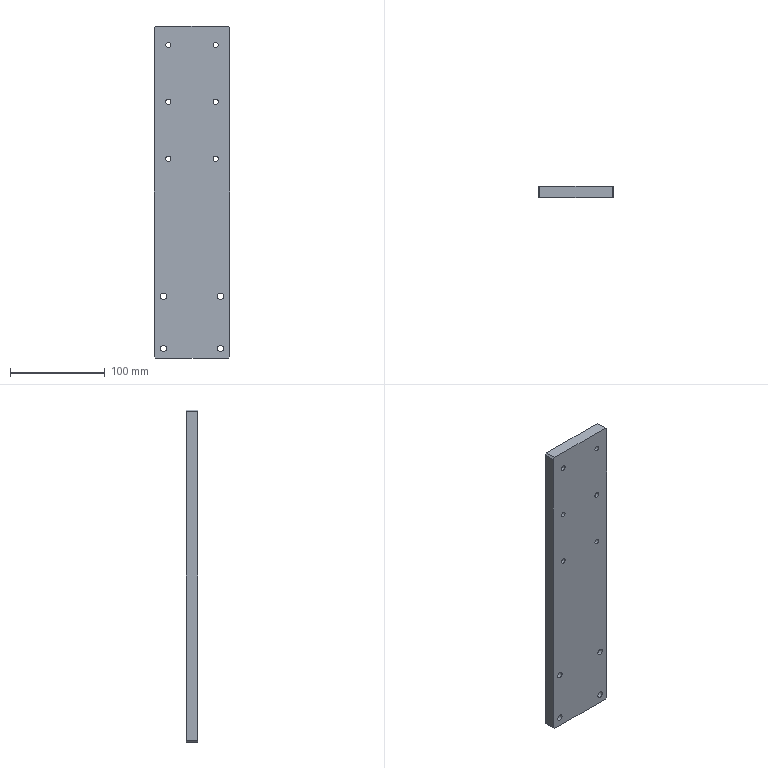Part | NX | 1 solid | 40 faces | box 80 x 12 x 350 mm | volume 329023 mm3 | plane 20 | cylinder 20 | commonest cylinder face diameters 5.5 x6 10 x6 6.6 x4 11 x4
STEP:
#1=CARTESIAN_POINT('',(40.,12.,173.));
#2=VERTEX_POINT('',#1);
#3=CARTESIAN_POINT('',(40.,12.,-173.));
#4=VERTEX_POINT('',#3);
#5=CARTESIAN_POINT('',(40.,12.,175.));
#6=DIRECTION('',(0.,0.,-1.));
#7=VECTOR('',#6,1000.);
#8=LINE('',#5,#7);
#9=EDGE_CURVE('',#2,#4,#8,.T.);
#10=ORIENTED_EDGE('',*,*,#9,.F.);
#11=CARTESIAN_POINT('',(40.,0.,173.));
#12=VERTEX_POINT('',#11);
#13=CARTESIAN_POINT('',(40.,12.,173.));
#14=DIRECTION('',(0.,-1.,0.));
#15=VECTOR('',#14,1000.);
#16=LINE('',#13,#15);
#17=EDGE_CURVE('',#2,#12,#16,.T.);
#18=ORIENTED_EDGE('',*,*,#17,.T.);
#19=CARTESIAN_POINT('',(40.,0.,-173.));
#20=VERTEX_POINT('',#19);
#21=CARTESIAN_POINT('',(40.,0.,175.));
#22=DIRECTION('',(0.,0.,-1.));
#23=VECTOR('',#22,1000.);
#24=LINE('',#21,#23);
#25=EDGE_CURVE('',#12,#20,#24,.T.);
#26=ORIENTED_EDGE('',*,*,#25,.T.);
#27=CARTESIAN_POINT('',(40.,12.,-173.));
#28=DIRECTION('',(0.,1.,0.));
#29=VECTOR('',#28,1000.);
#30=LINE('',#27,#29);
#31=EDGE_CURVE('',#20,#4,#30,.T.);
#32=ORIENTED_EDGE('',*,*,#31,.T.);
#33=EDGE_LOOP('',(#10,#18,#26,#32));
#34=FACE_BOUND('',#33,.T.);
#35=CARTESIAN_POINT('',(40.,12.,175.));
#36=DIRECTION('',(-1.,0.,0.));
#37=DIRECTION('',(0.,0.,1.));
#38=AXIS2_PLACEMENT_3D('',#35,#36,#37);
#39=PLANE('',#38);
#40=ADVANCED_FACE('',(#34),#39,.F.);
#41=CARTESIAN_POINT('',(38.,12.,-175.));
#42=VERTEX_POINT('',#41);
#43=CARTESIAN_POINT('',(-38.,12.,-175.));
#44=VERTEX_POINT('',#43);
#45=CARTESIAN_POINT('',(-40.,12.,-175.));
#46=DIRECTION('',(-1.,0.,0.));
#47=VECTOR('',#46,1000.);
#48=LINE('',#45,#47);
#49=EDGE_CURVE('',#42,#44,#48,.T.);
#50=ORIENTED_EDGE('',*,*,#49,.F.);
#51=CARTESIAN_POINT('',(38.,0.,-175.));
#52=VERTEX_POINT('',#51);
#53=CARTESIAN_POINT('',(38.,12.,-175.));
#54=DIRECTION('',(0.,-1.,0.));
#55=VECTOR('',#54,1000.);
#56=LINE('',#53,#55);
#57=EDGE_CURVE('',#42,#52,#56,.T.);
#58=ORIENTED_EDGE('',*,*,#57,.T.);
#59=CARTESIAN_POINT('',(-38.,0.,-175.));
#60=VERTEX_POINT('',#59);
#61=CARTESIAN_POINT('',(-40.,0.,-175.));
#62=DIRECTION('',(-1.,0.,0.));
#63=VECTOR('',#62,1000.);
#64=LINE('',#61,#63);
#65=EDGE_CURVE('',#52,#60,#64,.T.);
#66=ORIENTED_EDGE('',*,*,#65,.T.);
#67=CARTESIAN_POINT('',(-38.,12.,-175.));
#68=DIRECTION('',(0.,1.,0.));
#69=VECTOR('',#68,1000.);
#70=LINE('',#67,#69);
#71=EDGE_CURVE('',#60,#44,#70,.T.);
#72=ORIENTED_EDGE('',*,*,#71,.T.);
#73=EDGE_LOOP('',(#50,#58,#66,#72));
#74=FACE_BOUND('',#73,.T.);
#75=CARTESIAN_POINT('',(-40.,12.,-175.));
#76=DIRECTION('',(0.,0.,1.));
#77=DIRECTION('',(1.,0.,0.));
#78=AXIS2_PLACEMENT_3D('',#75,#76,#77);
#79=PLANE('',#78);
#80=ADVANCED_FACE('',(#74),#79,.F.);
#81=CARTESIAN_POINT('',(-40.,0.,-173.));
#82=VERTEX_POINT('',#81);
#83=CARTESIAN_POINT('',(-40.,0.,173.));
#84=VERTEX_POINT('',#83);
#85=CARTESIAN_POINT('',(-40.,0.,175.));
#86=DIRECTION('',(0.,0.,1.));
#87=VECTOR('',#86,1000.);
#88=LINE('',#85,#87);
#89=EDGE_CURVE('',#82,#84,#88,.T.);
#90=ORIENTED_EDGE('',*,*,#89,.T.);
#91=CARTESIAN_POINT('',(-40.,12.,173.));
#92=VERTEX_POINT('',#91);
#93=CARTESIAN_POINT('',(-40.,12.,173.));
#94=DIRECTION('',(0.,1.,0.));
#95=VECTOR('',#94,1000.);
#96=LINE('',#93,#95);
#97=EDGE_CURVE('',#84,#92,#96,.T.);
#98=ORIENTED_EDGE('',*,*,#97,.T.);
#99=CARTESIAN_POINT('',(-40.,12.,-173.));
#100=VERTEX_POINT('',#99);
#101=CARTESIAN_POINT('',(-40.,12.,175.));
#102=DIRECTION('',(0.,0.,1.));
#103=VECTOR('',#102,1000.);
#104=LINE('',#101,#103);
#105=EDGE_CURVE('',#100,#92,#104,.T.);
#106=ORIENTED_EDGE('',*,*,#105,.F.);
#107=CARTESIAN_POINT('',(-40.,12.,-173.));
#108=DIRECTION('',(0.,-1.,0.));
#109=VECTOR('',#108,1000.);
#110=LINE('',#107,#109);
#111=EDGE_CURVE('',#100,#82,#110,.T.);
#112=ORIENTED_EDGE('',*,*,#111,.T.);
#113=EDGE_LOOP('',(#90,#98,#106,#112));
#114=FACE_BOUND('',#113,.T.);
#115=CARTESIAN_POINT('',(-40.,12.,175.));
#116=DIRECTION('',(1.,0.,0.));
#117=DIRECTION('',(0.,0.,-1.));
#118=AXIS2_PLACEMENT_3D('',#115,#116,#117);
#119=PLANE('',#118);
#120=ADVANCED_FACE('',(#114),#119,.F.);
#121=CARTESIAN_POINT('',(-38.,12.,175.));
#122=VERTEX_POINT('',#121);
#123=CARTESIAN_POINT('',(38.,12.,175.));
#124=VERTEX_POINT('',#123);
#125=CARTESIAN_POINT('',(-40.,12.,175.));
#126=DIRECTION('',(1.,0.,0.));
#127=VECTOR('',#126,1000.);
#128=LINE('',#125,#127);
#129=EDGE_CURVE('',#122,#124,#128,.T.);
#130=ORIENTED_EDGE('',*,*,#129,.F.);
#131=CARTESIAN_POINT('',(-38.,0.,175.));
#132=VERTEX_POINT('',#131);
#133=CARTESIAN_POINT('',(-38.,12.,175.));
#134=DIRECTION('',(0.,-1.,0.));
#135=VECTOR('',#134,1000.);
#136=LINE('',#133,#135);
#137=EDGE_CURVE('',#122,#132,#136,.T.);
#138=ORIENTED_EDGE('',*,*,#137,.T.);
#139=CARTESIAN_POINT('',(38.,0.,175.));
#140=VERTEX_POINT('',#139);
#141=CARTESIAN_POINT('',(-40.,0.,175.));
#142=DIRECTION('',(1.,0.,0.));
#143=VECTOR('',#142,1000.);
#144=LINE('',#141,#143);
#145=EDGE_CURVE('',#132,#140,#144,.T.);
#146=ORIENTED_EDGE('',*,*,#145,.T.);
#147=CARTESIAN_POINT('',(38.,12.,175.));
#148=DIRECTION('',(0.,1.,0.));
#149=VECTOR('',#148,1000.);
#150=LINE('',#147,#149);
#151=EDGE_CURVE('',#140,#124,#150,.T.);
#152=ORIENTED_EDGE('',*,*,#151,.T.);
#153=EDGE_LOOP('',(#130,#138,#146,#152));
#154=FACE_BOUND('',#153,.T.);
#155=CARTESIAN_POINT('',(-40.,12.,175.));
#156=DIRECTION('',(0.,0.,-1.));
#157=DIRECTION('',(-1.,0.,0.));
#158=AXIS2_PLACEMENT_3D('',#155,#156,#157);
#159=PLANE('',#158);
#160=ADVANCED_FACE('',(#154),#159,.F.);
#161=CARTESIAN_POINT('',(-25.,12.,100.));
#162=VERTEX_POINT('',#161);
#163=CARTESIAN_POINT('',(-25.,12.,95.));
#164=DIRECTION('',(0.,1.,0.));
#165=DIRECTION('',(0.,0.,1.));
#166=AXIS2_PLACEMENT_3D('',#163,#164,#165);
#167=CIRCLE('',#166,5.);
#168=EDGE_CURVE('',#162,#162,#167,.T.);
#169=ORIENTED_EDGE('',*,*,#168,.F.);
#170=EDGE_LOOP('',(#169));
#171=FACE_BOUND('',#170,.T.);
#172=CARTESIAN_POINT('',(25.,12.,100.));
#173=VERTEX_POINT('',#172);
#174=CARTESIAN_POINT('',(25.,12.,95.));
#175=DIRECTION('',(0.,1.,0.));
#176=DIRECTION('',(0.,0.,1.));
#177=AXIS2_PLACEMENT_3D('',#174,#175,#176);
#178=CIRCLE('',#177,5.);
#179=EDGE_CURVE('',#173,#173,#178,.T.);
#180=ORIENTED_EDGE('',*,*,#179,.F.);
#181=EDGE_LOOP('',(#180));
#182=FACE_BOUND('',#181,.T.);
#183=CARTESIAN_POINT('',(25.,12.,160.));
#184=VERTEX_POINT('',#183);
#185=CARTESIAN_POINT('',(25.,12.,155.));
#186=DIRECTION('',(0.,1.,0.));
#187=DIRECTION('',(0.,0.,1.));
#188=AXIS2_PLACEMENT_3D('',#185,#186,#187);
#189=CIRCLE('',#188,5.);
#190=EDGE_CURVE('',#184,#184,#189,.T.);
#191=ORIENTED_EDGE('',*,*,#190,.F.);
#192=EDGE_LOOP('',(#191));
#193=FACE_BOUND('',#192,.T.);
#194=CARTESIAN_POINT('',(-25.,12.,160.));
#195=VERTEX_POINT('',#194);
#196=CARTESIAN_POINT('',(-25.,12.,155.));
#197=DIRECTION('',(0.,1.,0.));
#198=DIRECTION('',(0.,0.,1.));
#199=AXIS2_PLACEMENT_3D('',#196,#197,#198);
#200=CIRCLE('',#199,5.);
#201=EDGE_CURVE('',#195,#195,#200,.T.);
#202=ORIENTED_EDGE('',*,*,#201,.F.);
#203=EDGE_LOOP('',(#202));
#204=FACE_BOUND('',#203,.T.);
#205=CARTESIAN_POINT('',(-30.,12.,-159.5));
#206=VERTEX_POINT('',#205);
#207=CARTESIAN_POINT('',(-30.,12.,-165.));
#208=DIRECTION('',(0.,1.,0.));
#209=DIRECTION('',(0.,0.,1.));
#210=AXIS2_PLACEMENT_3D('',#207,#208,#209);
#211=CIRCLE('',#210,5.5);
#212=EDGE_CURVE('',#206,#206,#211,.T.);
#213=ORIENTED_EDGE('',*,*,#212,.F.);
#214=EDGE_LOOP('',(#213));
#215=FACE_BOUND('',#214,.T.);
#216=CARTESIAN_POINT('',(30.,12.,-159.5));
#217=VERTEX_POINT('',#216);
#218=CARTESIAN_POINT('',(30.,12.,-165.));
#219=DIRECTION('',(0.,1.,0.));
#220=DIRECTION('',(0.,0.,1.));
#221=AXIS2_PLACEMENT_3D('',#218,#219,#220);
#222=CIRCLE('',#221,5.5);
#223=EDGE_CURVE('',#217,#217,#222,.T.);
#224=ORIENTED_EDGE('',*,*,#223,.F.);
#225=EDGE_LOOP('',(#224));
#226=FACE_BOUND('',#225,.T.);
#227=CARTESIAN_POINT('',(-30.,12.,-104.5));
#228=VERTEX_POINT('',#227);
#229=CARTESIAN_POINT('',(-30.,12.,-110.));
#230=DIRECTION('',(0.,1.,0.));
#231=DIRECTION('',(0.,0.,1.));
#232=AXIS2_PLACEMENT_3D('',#229,#230,#231);
#233=CIRCLE('',#232,5.5);
#234=EDGE_CURVE('',#228,#228,#233,.T.);
#235=ORIENTED_EDGE('',*,*,#234,.F.);
#236=EDGE_LOOP('',(#235));
#237=FACE_BOUND('',#236,.T.);
#238=CARTESIAN_POINT('',(30.,12.,-104.5));
#239=VERTEX_POINT('',#238);
#240=CARTESIAN_POINT('',(30.,12.,-110.));
#241=DIRECTION('',(0.,1.,0.));
#242=DIRECTION('',(0.,0.,1.));
#243=AXIS2_PLACEMENT_3D('',#240,#241,#242);
#244=CIRCLE('',#243,5.5);
#245=EDGE_CURVE('',#239,#239,#244,.T.);
#246=ORIENTED_EDGE('',*,*,#245,.F.);
#247=EDGE_LOOP('',(#246));
#248=FACE_BOUND('',#247,.T.);
#249=ORIENTED_EDGE('',*,*,#105,.T.);
#250=CARTESIAN_POINT('',(-38.,12.,175.));
#251=DIRECTION('',(-0.7071,0.,-0.7071));
#252=VECTOR('',#251,1000.);
#253=LINE('',#250,#252);
#254=EDGE_CURVE('',#92,#122,#253,.F.);
#255=ORIENTED_EDGE('',*,*,#254,.T.);
#256=ORIENTED_EDGE('',*,*,#129,.T.);
#257=CARTESIAN_POINT('',(40.,12.,173.));
#258=DIRECTION('',(-0.7071,0.,0.7071));
#259=VECTOR('',#258,1000.);
#260=LINE('',#257,#259);
#261=EDGE_CURVE('',#124,#2,#260,.F.);
#262=ORIENTED_EDGE('',*,*,#261,.T.);
#263=ORIENTED_EDGE('',*,*,#9,.T.);
#264=CARTESIAN_POINT('',(38.,12.,-175.));
#265=DIRECTION('',(0.7071,0.,0.7071));
#266=VECTOR('',#265,1000.);
#267=LINE('',#264,#266);
#268=EDGE_CURVE('',#4,#42,#267,.F.);
#269=ORIENTED_EDGE('',*,*,#268,.T.);
#270=ORIENTED_EDGE('',*,*,#49,.T.);
#271=CARTESIAN_POINT('',(-40.,12.,-173.));
#272=DIRECTION('',(0.7071,0.,-0.7071));
#273=VECTOR('',#272,1000.);
#274=LINE('',#271,#273);
#275=EDGE_CURVE('',#44,#100,#274,.F.);
#276=ORIENTED_EDGE('',*,*,#275,.T.);
#277=EDGE_LOOP('',(#249,#255,#256,#262,#263,#269,#270,#276));
#278=FACE_BOUND('',#277,.T.);
#279=CARTESIAN_POINT('',(25.,12.,40.));
#280=VERTEX_POINT('',#279);
#281=CARTESIAN_POINT('',(25.,12.,35.));
#282=DIRECTION('',(0.,1.,0.));
#283=DIRECTION('',(0.,0.,1.));
#284=AXIS2_PLACEMENT_3D('',#281,#282,#283);
#285=CIRCLE('',#284,5.);
#286=EDGE_CURVE('',#280,#280,#285,.T.);
#287=ORIENTED_EDGE('',*,*,#286,.F.);
#288=EDGE_LOOP('',(#287));
#289=FACE_BOUND('',#288,.T.);
#290=CARTESIAN_POINT('',(-25.,12.,40.));
#291=VERTEX_POINT('',#290);
#292=CARTESIAN_POINT('',(-25.,12.,35.));
#293=DIRECTION('',(0.,1.,0.));
#294=DIRECTION('',(0.,0.,1.));
#295=AXIS2_PLACEMENT_3D('',#292,#293,#294);
#296=CIRCLE('',#295,5.);
#297=EDGE_CURVE('',#291,#291,#296,.T.);
#298=ORIENTED_EDGE('',*,*,#297,.F.);
#299=EDGE_LOOP('',(#298));
#300=FACE_BOUND('',#299,.T.);
#301=CARTESIAN_POINT('',(0.,12.,0.));
#302=DIRECTION('',(0.,-1.,0.));
#303=DIRECTION('',(0.,0.,-1.));
#304=AXIS2_PLACEMENT_3D('',#301,#302,#303);
#305=PLANE('',#304);
#306=ADVANCED_FACE('',(#171,#182,#193,#204,#215,#226,#237,#248,#278,#289,#300),#305,.F.);
#307=CARTESIAN_POINT('',(-25.,0.,97.75));
#308=VERTEX_POINT('',#307);
#309=CARTESIAN_POINT('',(-25.,0.,95.));
#310=DIRECTION('',(0.,1.,0.));
#311=DIRECTION('',(0.,0.,1.));
#312=AXIS2_PLACEMENT_3D('',#309,#310,#311);
#313=CIRCLE('',#312,2.75);
#314=EDGE_CURVE('',#308,#308,#313,.T.);
#315=ORIENTED_EDGE('',*,*,#314,.T.);
#316=EDGE_LOOP('',(#315));
#317=FACE_BOUND('',#316,.T.);
#318=CARTESIAN_POINT('',(25.,0.,97.75));
#319=VERTEX_POINT('',#318);
#320=CARTESIAN_POINT('',(25.,0.,95.));
#321=DIRECTION('',(0.,1.,0.));
#322=DIRECTION('',(0.,0.,1.));
#323=AXIS2_PLACEMENT_3D('',#320,#321,#322);
#324=CIRCLE('',#323,2.75);
#325=EDGE_CURVE('',#319,#319,#324,.T.);
#326=ORIENTED_EDGE('',*,*,#325,.T.);
#327=EDGE_LOOP('',(#326));
#328=FACE_BOUND('',#327,.T.);
#329=CARTESIAN_POINT('',(25.,0.,157.75));
#330=VERTEX_POINT('',#329);
#331=CARTESIAN_POINT('',(25.,0.,155.));
#332=DIRECTION('',(0.,1.,0.));
#333=DIRECTION('',(0.,0.,1.));
#334=AXIS2_PLACEMENT_3D('',#331,#332,#333);
#335=CIRCLE('',#334,2.75);
#336=EDGE_CURVE('',#330,#330,#335,.T.);
#337=ORIENTED_EDGE('',*,*,#336,.T.);
#338=EDGE_LOOP('',(#337));
#339=FACE_BOUND('',#338,.T.);
#340=CARTESIAN_POINT('',(-25.,0.,157.75));
#341=VERTEX_POINT('',#340);
#342=CARTESIAN_POINT('',(-25.,0.,155.));
#343=DIRECTION('',(0.,1.,0.));
#344=DIRECTION('',(0.,0.,1.));
#345=AXIS2_PLACEMENT_3D('',#342,#343,#344);
#346=CIRCLE('',#345,2.75);
#347=EDGE_CURVE('',#341,#341,#346,.T.);
#348=ORIENTED_EDGE('',*,*,#347,.T.);
#349=EDGE_LOOP('',(#348));
#350=FACE_BOUND('',#349,.T.);
#351=CARTESIAN_POINT('',(-30.,0.,-161.7));
#352=VERTEX_POINT('',#351);
#353=CARTESIAN_POINT('',(-30.,0.,-165.));
#354=DIRECTION('',(0.,1.,0.));
#355=DIRECTION('',(0.,0.,1.));
#356=AXIS2_PLACEMENT_3D('',#353,#354,#355);
#357=CIRCLE('',#356,3.3);
#358=EDGE_CURVE('',#352,#352,#357,.T.);
#359=ORIENTED_EDGE('',*,*,#358,.T.);
#360=EDGE_LOOP('',(#359));
#361=FACE_BOUND('',#360,.T.);
#362=CARTESIAN_POINT('',(30.,0.,-161.7));
#363=VERTEX_POINT('',#362);
#364=CARTESIAN_POINT('',(30.,0.,-165.));
#365=DIRECTION('',(0.,1.,0.));
#366=DIRECTION('',(0.,0.,1.));
#367=AXIS2_PLACEMENT_3D('',#364,#365,#366);
#368=CIRCLE('',#367,3.3);
#369=EDGE_CURVE('',#363,#363,#368,.T.);
#370=ORIENTED_EDGE('',*,*,#369,.T.);
#371=EDGE_LOOP('',(#370));
#372=FACE_BOUND('',#371,.T.);
#373=CARTESIAN_POINT('',(-30.,0.,-106.7));
#374=VERTEX_POINT('',#373);
#375=CARTESIAN_POINT('',(-30.,0.,-110.));
#376=DIRECTION('',(0.,1.,0.));
#377=DIRECTION('',(0.,0.,1.));
#378=AXIS2_PLACEMENT_3D('',#375,#376,#377);
#379=CIRCLE('',#378,3.3);
#380=EDGE_CURVE('',#374,#374,#379,.T.);
#381=ORIENTED_EDGE('',*,*,#380,.T.);
#382=EDGE_LOOP('',(#381));
#383=FACE_BOUND('',#382,.T.);
#384=CARTESIAN_POINT('',(30.,0.,-106.7));
#385=VERTEX_POINT('',#384);
#386=CARTESIAN_POINT('',(30.,0.,-110.));
#387=DIRECTION('',(0.,1.,0.));
#388=DIRECTION('',(0.,0.,1.));
#389=AXIS2_PLACEMENT_3D('',#386,#387,#388);
#390=CIRCLE('',#389,3.3);
#391=EDGE_CURVE('',#385,#385,#390,.T.);
#392=ORIENTED_EDGE('',*,*,#391,.T.);
#393=EDGE_LOOP('',(#392));
#394=FACE_BOUND('',#393,.T.);
#395=ORIENTED_EDGE('',*,*,#145,.F.);
#396=CARTESIAN_POINT('',(-106.5,0.,106.5));
#397=DIRECTION('',(0.7071,0.,0.7071));
#398=VECTOR('',#397,1000.);
#399=LINE('',#396,#398);
#400=EDGE_CURVE('',#132,#84,#399,.F.);
#401=ORIENTED_EDGE('',*,*,#400,.T.);
#402=ORIENTED_EDGE('',*,*,#89,.F.);
#403=CARTESIAN_POINT('',(-106.5,0.,-106.5));
#404=DIRECTION('',(-0.7071,0.,0.7071));
#405=VECTOR('',#404,1000.);
#406=LINE('',#403,#405);
#407=EDGE_CURVE('',#82,#60,#406,.F.);
#408=ORIENTED_EDGE('',*,*,#407,.T.);
#409=ORIENTED_EDGE('',*,*,#65,.F.);
#410=CARTESIAN_POINT('',(106.5,0.,-106.5));
#411=DIRECTION('',(-0.7071,0.,-0.7071));
#412=VECTOR('',#411,1000.);
#413=LINE('',#410,#412);
#414=EDGE_CURVE('',#52,#20,#413,.F.);
#415=ORIENTED_EDGE('',*,*,#414,.T.);
#416=ORIENTED_EDGE('',*,*,#25,.F.);
#417=CARTESIAN_POINT('',(106.5,0.,106.5));
#418=DIRECTION('',(0.7071,0.,-0.7071));
#419=VECTOR('',#418,1000.);
#420=LINE('',#417,#419);
#421=EDGE_CURVE('',#12,#140,#420,.F.);
#422=ORIENTED_EDGE('',*,*,#421,.T.);
#423=EDGE_LOOP('',(#395,#401,#402,#408,#409,#415,#416,#422));
#424=FACE_BOUND('',#423,.T.);
#425=CARTESIAN_POINT('',(25.,0.,37.75));
#426=VERTEX_POINT('',#425);
#427=CARTESIAN_POINT('',(25.,0.,35.));
#428=DIRECTION('',(0.,1.,0.));
#429=DIRECTION('',(0.,0.,1.));
#430=AXIS2_PLACEMENT_3D('',#427,#428,#429);
#431=CIRCLE('',#430,2.75);
#432=EDGE_CURVE('',#426,#426,#431,.T.);
#433=ORIENTED_EDGE('',*,*,#432,.T.);
#434=EDGE_LOOP('',(#433));
#435=FACE_BOUND('',#434,.T.);
#436=CARTESIAN_POINT('',(-25.,0.,37.75));
#437=VERTEX_POINT('',#436);
#438=CARTESIAN_POINT('',(-25.,0.,35.));
#439=DIRECTION('',(0.,1.,0.));
#440=DIRECTION('',(0.,0.,1.));
#441=AXIS2_PLACEMENT_3D('',#438,#439,#440);
#442=CIRCLE('',#441,2.75);
#443=EDGE_CURVE('',#437,#437,#442,.T.);
#444=ORIENTED_EDGE('',*,*,#443,.T.);
#445=EDGE_LOOP('',(#444));
#446=FACE_BOUND('',#445,.T.);
#447=CARTESIAN_POINT('',(0.,0.,0.));
#448=DIRECTION('',(0.,-1.,0.));
#449=DIRECTION('',(0.,0.,-1.));
#450=AXIS2_PLACEMENT_3D('',#447,#448,#449);
#451=PLANE('',#450);
#452=ADVANCED_FACE('',(#317,#328,#339,#350,#361,#372,#383,#394,#424,#435,#446),#451,.T.);
#453=ORIENTED_EDGE('',*,*,#254,.F.);
#454=ORIENTED_EDGE('',*,*,#97,.F.);
#455=ORIENTED_EDGE('',*,*,#400,.F.);
#456=ORIENTED_EDGE('',*,*,#137,.F.);
#457=EDGE_LOOP('',(#453,#454,#455,#456));
#458=FACE_BOUND('',#457,.T.);
#459=CARTESIAN_POINT('',(-38.,12.,175.));
#460=DIRECTION('',(0.7071,0.,-0.7071));
#461=DIRECTION('',(0.,-1.,0.));
#462=AXIS2_PLACEMENT_3D('',#459,#460,#461);
#463=PLANE('',#462);
#464=ADVANCED_FACE('',(#458),#463,.F.);
#465=ORIENTED_EDGE('',*,*,#261,.F.);
#466=ORIENTED_EDGE('',*,*,#151,.F.);
#467=ORIENTED_EDGE('',*,*,#421,.F.);
#468=ORIENTED_EDGE('',*,*,#17,.F.);
#469=EDGE_LOOP('',(#465,#466,#467,#468));
#470=FACE_BOUND('',#469,.T.);
#471=CARTESIAN_POINT('',(40.,12.,173.));
#472=DIRECTION('',(-0.7071,0.,-0.7071));
#473=DIRECTION('',(0.,-1.,0.));
#474=AXIS2_PLACEMENT_3D('',#471,#472,#473);
#475=PLANE('',#474);
#476=ADVANCED_FACE('',(#470),#475,.F.);
#477=ORIENTED_EDGE('',*,*,#268,.F.);
#478=ORIENTED_EDGE('',*,*,#31,.F.);
#479=ORIENTED_EDGE('',*,*,#414,.F.);
#480=ORIENTED_EDGE('',*,*,#57,.F.);
#481=EDGE_LOOP('',(#477,#478,#479,#480));
#482=FACE_BOUND('',#481,.T.);
#483=CARTESIAN_POINT('',(38.,12.,-175.));
#484=DIRECTION('',(-0.7071,0.,0.7071));
#485=DIRECTION('',(0.,-1.,0.));
#486=AXIS2_PLACEMENT_3D('',#483,#484,#485);
#487=PLANE('',#486);
#488=ADVANCED_FACE('',(#482),#487,.F.);
#489=ORIENTED_EDGE('',*,*,#275,.F.);
#490=ORIENTED_EDGE('',*,*,#71,.F.);
#491=ORIENTED_EDGE('',*,*,#407,.F.);
#492=ORIENTED_EDGE('',*,*,#111,.F.);
#493=EDGE_LOOP('',(#489,#490,#491,#492));
#494=FACE_BOUND('',#493,.T.);
#495=CARTESIAN_POINT('',(-40.,12.,-173.));
#496=DIRECTION('',(0.7071,0.,0.7071));
#497=DIRECTION('',(0.,-1.,0.));
#498=AXIS2_PLACEMENT_3D('',#495,#496,#497);
#499=PLANE('',#498);
#500=ADVANCED_FACE('',(#494),#499,.F.);
#501=ORIENTED_EDGE('',*,*,#391,.F.);
#502=EDGE_LOOP('',(#501));
#503=FACE_BOUND('',#502,.T.);
#504=CARTESIAN_POINT('',(30.,5.2,-106.7));
#505=VERTEX_POINT('',#504);
#506=CARTESIAN_POINT('',(30.,5.2,-110.));
#507=DIRECTION('',(0.,1.,0.));
#508=DIRECTION('',(0.,0.,1.));
#509=AXIS2_PLACEMENT_3D('',#506,#507,#508);
#510=CIRCLE('',#509,3.3);
#511=EDGE_CURVE('',#505,#505,#510,.T.);
#512=ORIENTED_EDGE('',*,*,#511,.T.);
#513=EDGE_LOOP('',(#512));
#514=FACE_BOUND('',#513,.T.);
#515=CARTESIAN_POINT('',(30.,12.,-110.));
#516=DIRECTION('',(0.,1.,0.));
#517=DIRECTION('',(0.,0.,1.));
#518=AXIS2_PLACEMENT_3D('',#515,#516,#517);
#519=CYLINDRICAL_SURFACE('',#518,3.3);
#520=ADVANCED_FACE('',(#503,#514),#519,.F.);
#521=ORIENTED_EDGE('',*,*,#511,.F.);
#522=EDGE_LOOP('',(#521));
#523=FACE_BOUND('',#522,.T.);
#524=CARTESIAN_POINT('',(30.,5.2,-104.5));
#525=VERTEX_POINT('',#524);
#526=CARTESIAN_POINT('',(30.,5.2,-110.));
#527=DIRECTION('',(0.,1.,0.));
#528=DIRECTION('',(0.,0.,1.));
#529=AXIS2_PLACEMENT_3D('',#526,#527,#528);
#530=CIRCLE('',#529,5.5);
#531=EDGE_CURVE('',#525,#525,#530,.T.);
#532=ORIENTED_EDGE('',*,*,#531,.T.);
#533=EDGE_LOOP('',(#532));
#534=FACE_BOUND('',#533,.T.);
#535=CARTESIAN_POINT('',(33.3,5.2,-110.));
#536=DIRECTION('',(0.,-1.,0.));
#537=DIRECTION('',(0.,0.,-1.));
#538=AXIS2_PLACEMENT_3D('',#535,#536,#537);
#539=PLANE('',#538);
#540=ADVANCED_FACE('',(#523,#534),#539,.F.);
#541=ORIENTED_EDGE('',*,*,#531,.F.);
#542=EDGE_LOOP('',(#541));
#543=FACE_BOUND('',#542,.T.);
#544=ORIENTED_EDGE('',*,*,#245,.T.);
#545=EDGE_LOOP('',(#544));
#546=FACE_BOUND('',#545,.T.);
#547=CARTESIAN_POINT('',(30.,12.,-110.));
#548=DIRECTION('',(0.,1.,0.));
#549=DIRECTION('',(0.,0.,1.));
#550=AXIS2_PLACEMENT_3D('',#547,#548,#549);
#551=CYLINDRICAL_SURFACE('',#550,5.5);
#552=ADVANCED_FACE('',(#543,#546),#551,.F.);
#553=ORIENTED_EDGE('',*,*,#380,.F.);
#554=EDGE_LOOP('',(#553));
#555=FACE_BOUND('',#554,.T.);
#556=CARTESIAN_POINT('',(-30.,5.2,-106.7));
#557=VERTEX_POINT('',#556);
#558=CARTESIAN_POINT('',(-30.,5.2,-110.));
#559=DIRECTION('',(0.,1.,0.));
#560=DIRECTION('',(0.,0.,1.));
#561=AXIS2_PLACEMENT_3D('',#558,#559,#560);
#562=CIRCLE('',#561,3.3);
#563=EDGE_CURVE('',#557,#557,#562,.T.);
#564=ORIENTED_EDGE('',*,*,#563,.T.);
#565=EDGE_LOOP('',(#564));
#566=FACE_BOUND('',#565,.T.);
#567=CARTESIAN_POINT('',(-30.,12.,-110.));
#568=DIRECTION('',(0.,1.,0.));
#569=DIRECTION('',(0.,0.,1.));
#570=AXIS2_PLACEMENT_3D('',#567,#568,#569);
#571=CYLINDRICAL_SURFACE('',#570,3.3);
#572=ADVANCED_FACE('',(#555,#566),#571,.F.);
#573=ORIENTED_EDGE('',*,*,#563,.F.);
#574=EDGE_LOOP('',(#573));
#575=FACE_BOUND('',#574,.T.);
#576=CARTESIAN_POINT('',(-30.,5.2,-104.5));
#577=VERTEX_POINT('',#576);
#578=CARTESIAN_POINT('',(-30.,5.2,-110.));
#579=DIRECTION('',(0.,1.,0.));
#580=DIRECTION('',(0.,0.,1.));
#581=AXIS2_PLACEMENT_3D('',#578,#579,#580);
#582=CIRCLE('',#581,5.5);
#583=EDGE_CURVE('',#577,#577,#582,.T.);
#584=ORIENTED_EDGE('',*,*,#583,.T.);
#585=EDGE_LOOP('',(#584));
#586=FACE_BOUND('',#585,.T.);
#587=CARTESIAN_POINT('',(-26.7,5.2,-110.));
#588=DIRECTION('',(0.,-1.,0.));
#589=DIRECTION('',(0.,0.,-1.));
#590=AXIS2_PLACEMENT_3D('',#587,#588,#589);
#591=PLANE('',#590);
#592=ADVANCED_FACE('',(#575,#586),#591,.F.);
#593=ORIENTED_EDGE('',*,*,#583,.F.);
#594=EDGE_LOOP('',(#593));
#595=FACE_BOUND('',#594,.T.);
#596=ORIENTED_EDGE('',*,*,#234,.T.);
#597=EDGE_LOOP('',(#596));
#598=FACE_BOUND('',#597,.T.);
#599=CARTESIAN_POINT('',(-30.,12.,-110.));
#600=DIRECTION('',(0.,1.,0.));
#601=DIRECTION('',(0.,0.,1.));
#602=AXIS2_PLACEMENT_3D('',#599,#600,#601);
#603=CYLINDRICAL_SURFACE('',#602,5.5);
#604=ADVANCED_FACE('',(#595,#598),#603,.F.);
#605=ORIENTED_EDGE('',*,*,#369,.F.);
#606=EDGE_LOOP('',(#605));
#607=FACE_BOUND('',#606,.T.);
#608=CARTESIAN_POINT('',(30.,5.2,-161.7));
#609=VERTEX_POINT('',#608);
#610=CARTESIAN_POINT('',(30.,5.2,-165.));
#611=DIRECTION('',(0.,1.,0.));
#612=DIRECTION('',(0.,0.,1.));
#613=AXIS2_PLACEMENT_3D('',#610,#611,#612);
#614=CIRCLE('',#613,3.3);
#615=EDGE_CURVE('',#609,#609,#614,.T.);
#616=ORIENTED_EDGE('',*,*,#615,.T.);
#617=EDGE_LOOP('',(#616));
#618=FACE_BOUND('',#617,.T.);
#619=CARTESIAN_POINT('',(30.,12.,-165.));
#620=DIRECTION('',(0.,1.,0.));
#621=DIRECTION('',(0.,0.,1.));
#622=AXIS2_PLACEMENT_3D('',#619,#620,#621);
#623=CYLINDRICAL_SURFACE('',#622,3.3);
#624=ADVANCED_FACE('',(#607,#618),#623,.F.);
#625=ORIENTED_EDGE('',*,*,#615,.F.);
#626=EDGE_LOOP('',(#625));
#627=FACE_BOUND('',#626,.T.);
#628=CARTESIAN_POINT('',(30.,5.2,-159.5));
#629=VERTEX_POINT('',#628);
#630=CARTESIAN_POINT('',(30.,5.2,-165.));
#631=DIRECTION('',(0.,1.,0.));
#632=DIRECTION('',(0.,0.,1.));
#633=AXIS2_PLACEMENT_3D('',#630,#631,#632);
#634=CIRCLE('',#633,5.5);
#635=EDGE_CURVE('',#629,#629,#634,.T.);
#636=ORIENTED_EDGE('',*,*,#635,.T.);
#637=EDGE_LOOP('',(#636));
#638=FACE_BOUND('',#637,.T.);
#639=CARTESIAN_POINT('',(33.3,5.2,-165.));
#640=DIRECTION('',(0.,-1.,0.));
#641=DIRECTION('',(0.,0.,-1.));
#642=AXIS2_PLACEMENT_3D('',#639,#640,#641);
#643=PLANE('',#642);
#644=ADVANCED_FACE('',(#627,#638),#643,.F.);
#645=ORIENTED_EDGE('',*,*,#635,.F.);
#646=EDGE_LOOP('',(#645));
#647=FACE_BOUND('',#646,.T.);
#648=ORIENTED_EDGE('',*,*,#223,.T.);
#649=EDGE_LOOP('',(#648));
#650=FACE_BOUND('',#649,.T.);
#651=CARTESIAN_POINT('',(30.,12.,-165.));
#652=DIRECTION('',(0.,1.,0.));
#653=DIRECTION('',(0.,0.,1.));
#654=AXIS2_PLACEMENT_3D('',#651,#652,#653);
#655=CYLINDRICAL_SURFACE('',#654,5.5);
#656=ADVANCED_FACE('',(#647,#650),#655,.F.);
#657=ORIENTED_EDGE('',*,*,#358,.F.);
#658=EDGE_LOOP('',(#657));
#659=FACE_BOUND('',#658,.T.);
#660=CARTESIAN_POINT('',(-30.,5.2,-161.7));
#661=VERTEX_POINT('',#660);
#662=CARTESIAN_POINT('',(-30.,5.2,-165.));
#663=DIRECTION('',(0.,1.,0.));
#664=DIRECTION('',(0.,0.,1.));
#665=AXIS2_PLACEMENT_3D('',#662,#663,#664);
#666=CIRCLE('',#665,3.3);
#667=EDGE_CURVE('',#661,#661,#666,.T.);
#668=ORIENTED_EDGE('',*,*,#667,.T.);
#669=EDGE_LOOP('',(#668));
#670=FACE_BOUND('',#669,.T.);
#671=CARTESIAN_POINT('',(-30.,12.,-165.));
#672=DIRECTION('',(0.,1.,0.));
#673=DIRECTION('',(0.,0.,1.));
#674=AXIS2_PLACEMENT_3D('',#671,#672,#673);
#675=CYLINDRICAL_SURFACE('',#674,3.3);
#676=ADVANCED_FACE('',(#659,#670),#675,.F.);
#677=ORIENTED_EDGE('',*,*,#667,.F.);
#678=EDGE_LOOP('',(#677));
#679=FACE_BOUND('',#678,.T.);
#680=CARTESIAN_POINT('',(-30.,5.2,-159.5));
#681=VERTEX_POINT('',#680);
#682=CARTESIAN_POINT('',(-30.,5.2,-165.));
#683=DIRECTION('',(0.,1.,0.));
#684=DIRECTION('',(0.,0.,1.));
#685=AXIS2_PLACEMENT_3D('',#682,#683,#684);
#686=CIRCLE('',#685,5.5);
#687=EDGE_CURVE('',#681,#681,#686,.T.);
#688=ORIENTED_EDGE('',*,*,#687,.T.);
#689=EDGE_LOOP('',(#688));
#690=FACE_BOUND('',#689,.T.);
#691=CARTESIAN_POINT('',(-26.7,5.2,-165.));
#692=DIRECTION('',(0.,-1.,0.));
#693=DIRECTION('',(0.,0.,-1.));
#694=AXIS2_PLACEMENT_3D('',#691,#692,#693);
#695=PLANE('',#694);
#696=ADVANCED_FACE('',(#679,#690),#695,.F.);
#697=ORIENTED_EDGE('',*,*,#687,.F.);
#698=EDGE_LOOP('',(#697));
#699=FACE_BOUND('',#698,.T.);
#700=ORIENTED_EDGE('',*,*,#212,.T.);
#701=EDGE_LOOP('',(#700));
#702=FACE_BOUND('',#701,.T.);
#703=CARTESIAN_POINT('',(-30.,12.,-165.));
#704=DIRECTION('',(0.,1.,0.));
#705=DIRECTION('',(0.,0.,1.));
#706=AXIS2_PLACEMENT_3D('',#703,#704,#705);
#707=CYLINDRICAL_SURFACE('',#706,5.5);
#708=ADVANCED_FACE('',(#699,#702),#707,.F.);
#709=ORIENTED_EDGE('',*,*,#347,.F.);
#710=EDGE_LOOP('',(#709));
#711=FACE_BOUND('',#710,.T.);
#712=CARTESIAN_POINT('',(-25.,6.3,157.75));
#713=VERTEX_POINT('',#712);
#714=CARTESIAN_POINT('',(-25.,6.3,155.));
#715=DIRECTION('',(0.,1.,0.));
#716=DIRECTION('',(0.,0.,1.));
#717=AXIS2_PLACEMENT_3D('',#714,#715,#716);
#718=CIRCLE('',#717,2.75);
#719=EDGE_CURVE('',#713,#713,#718,.T.);
#720=ORIENTED_EDGE('',*,*,#719,.T.);
#721=EDGE_LOOP('',(#720));
#722=FACE_BOUND('',#721,.T.);
#723=CARTESIAN_POINT('',(-25.,12.,155.));
#724=DIRECTION('',(0.,1.,0.));
#725=DIRECTION('',(0.,0.,1.));
#726=AXIS2_PLACEMENT_3D('',#723,#724,#725);
#727=CYLINDRICAL_SURFACE('',#726,2.75);
#728=ADVANCED_FACE('',(#711,#722),#727,.F.);
#729=ORIENTED_EDGE('',*,*,#719,.F.);
#730=EDGE_LOOP('',(#729));
#731=FACE_BOUND('',#730,.T.);
#732=CARTESIAN_POINT('',(-25.,6.3,160.));
#733=VERTEX_POINT('',#732);
#734=CARTESIAN_POINT('',(-25.,6.3,155.));
#735=DIRECTION('',(0.,1.,0.));
#736=DIRECTION('',(0.,0.,1.));
#737=AXIS2_PLACEMENT_3D('',#734,#735,#736);
#738=CIRCLE('',#737,5.);
#739=EDGE_CURVE('',#733,#733,#738,.T.);
#740=ORIENTED_EDGE('',*,*,#739,.T.);
#741=EDGE_LOOP('',(#740));
#742=FACE_BOUND('',#741,.T.);
#743=CARTESIAN_POINT('',(-22.25,6.3,155.));
#744=DIRECTION('',(0.,-1.,0.));
#745=DIRECTION('',(0.,0.,-1.));
#746=AXIS2_PLACEMENT_3D('',#743,#744,#745);
#747=PLANE('',#746);
#748=ADVANCED_FACE('',(#731,#742),#747,.F.);
#749=ORIENTED_EDGE('',*,*,#739,.F.);
#750=EDGE_LOOP('',(#749));
#751=FACE_BOUND('',#750,.T.);
#752=ORIENTED_EDGE('',*,*,#201,.T.);
#753=EDGE_LOOP('',(#752));
#754=FACE_BOUND('',#753,.T.);
#755=CARTESIAN_POINT('',(-25.,12.,155.));
#756=DIRECTION('',(0.,1.,0.));
#757=DIRECTION('',(0.,0.,1.));
#758=AXIS2_PLACEMENT_3D('',#755,#756,#757);
#759=CYLINDRICAL_SURFACE('',#758,5.);
#760=ADVANCED_FACE('',(#751,#754),#759,.F.);
#761=ORIENTED_EDGE('',*,*,#336,.F.);
#762=EDGE_LOOP('',(#761));
#763=FACE_BOUND('',#762,.T.);
#764=CARTESIAN_POINT('',(25.,6.3,157.75));
#765=VERTEX_POINT('',#764);
#766=CARTESIAN_POINT('',(25.,6.3,155.));
#767=DIRECTION('',(0.,1.,0.));
#768=DIRECTION('',(0.,0.,1.));
#769=AXIS2_PLACEMENT_3D('',#766,#767,#768);
#770=CIRCLE('',#769,2.75);
#771=EDGE_CURVE('',#765,#765,#770,.T.);
#772=ORIENTED_EDGE('',*,*,#771,.T.);
#773=EDGE_LOOP('',(#772));
#774=FACE_BOUND('',#773,.T.);
#775=CARTESIAN_POINT('',(25.,12.,155.));
#776=DIRECTION('',(0.,1.,0.));
#777=DIRECTION('',(0.,0.,1.));
#778=AXIS2_PLACEMENT_3D('',#775,#776,#777);
#779=CYLINDRICAL_SURFACE('',#778,2.75);
#780=ADVANCED_FACE('',(#763,#774),#779,.F.);
#781=ORIENTED_EDGE('',*,*,#771,.F.);
#782=EDGE_LOOP('',(#781));
#783=FACE_BOUND('',#782,.T.);
#784=CARTESIAN_POINT('',(25.,6.3,160.));
#785=VERTEX_POINT('',#784);
#786=CARTESIAN_POINT('',(25.,6.3,155.));
#787=DIRECTION('',(0.,1.,0.));
#788=DIRECTION('',(0.,0.,1.));
#789=AXIS2_PLACEMENT_3D('',#786,#787,#788);
#790=CIRCLE('',#789,5.);
#791=EDGE_CURVE('',#785,#785,#790,.T.);
#792=ORIENTED_EDGE('',*,*,#791,.T.);
#793=EDGE_LOOP('',(#792));
#794=FACE_BOUND('',#793,.T.);
#795=CARTESIAN_POINT('',(27.75,6.3,155.));
#796=DIRECTION('',(0.,-1.,0.));
#797=DIRECTION('',(0.,0.,-1.));
#798=AXIS2_PLACEMENT_3D('',#795,#796,#797);
#799=PLANE('',#798);
#800=ADVANCED_FACE('',(#783,#794),#799,.F.);
#801=ORIENTED_EDGE('',*,*,#791,.F.);
#802=EDGE_LOOP('',(#801));
#803=FACE_BOUND('',#802,.T.);
#804=ORIENTED_EDGE('',*,*,#190,.T.);
#805=EDGE_LOOP('',(#804));
#806=FACE_BOUND('',#805,.T.);
#807=CARTESIAN_POINT('',(25.,12.,155.));
#808=DIRECTION('',(0.,1.,0.));
#809=DIRECTION('',(0.,0.,1.));
#810=AXIS2_PLACEMENT_3D('',#807,#808,#809);
#811=CYLINDRICAL_SURFACE('',#810,5.);
#812=ADVANCED_FACE('',(#803,#806),#811,.F.);
#813=ORIENTED_EDGE('',*,*,#325,.F.);
#814=EDGE_LOOP('',(#813));
#815=FACE_BOUND('',#814,.T.);
#816=CARTESIAN_POINT('',(25.,6.3,97.75));
#817=VERTEX_POINT('',#816);
#818=CARTESIAN_POINT('',(25.,6.3,95.));
#819=DIRECTION('',(0.,1.,0.));
#820=DIRECTION('',(0.,0.,1.));
#821=AXIS2_PLACEMENT_3D('',#818,#819,#820);
#822=CIRCLE('',#821,2.75);
#823=EDGE_CURVE('',#817,#817,#822,.T.);
#824=ORIENTED_EDGE('',*,*,#823,.T.);
#825=EDGE_LOOP('',(#824));
#826=FACE_BOUND('',#825,.T.);
#827=CARTESIAN_POINT('',(25.,12.,95.));
#828=DIRECTION('',(0.,1.,0.));
#829=DIRECTION('',(0.,0.,1.));
#830=AXIS2_PLACEMENT_3D('',#827,#828,#829);
#831=CYLINDRICAL_SURFACE('',#830,2.75);
#832=ADVANCED_FACE('',(#815,#826),#831,.F.);
#833=ORIENTED_EDGE('',*,*,#823,.F.);
#834=EDGE_LOOP('',(#833));
#835=FACE_BOUND('',#834,.T.);
#836=CARTESIAN_POINT('',(25.,6.3,100.));
#837=VERTEX_POINT('',#836);
#838=CARTESIAN_POINT('',(25.,6.3,95.));
#839=DIRECTION('',(0.,1.,0.));
#840=DIRECTION('',(0.,0.,1.));
#841=AXIS2_PLACEMENT_3D('',#838,#839,#840);
#842=CIRCLE('',#841,5.);
#843=EDGE_CURVE('',#837,#837,#842,.T.);
#844=ORIENTED_EDGE('',*,*,#843,.T.);
#845=EDGE_LOOP('',(#844));
#846=FACE_BOUND('',#845,.T.);
#847=CARTESIAN_POINT('',(27.75,6.3,95.));
#848=DIRECTION('',(0.,-1.,0.));
#849=DIRECTION('',(0.,0.,-1.));
#850=AXIS2_PLACEMENT_3D('',#847,#848,#849);
#851=PLANE('',#850);
#852=ADVANCED_FACE('',(#835,#846),#851,.F.);
#853=ORIENTED_EDGE('',*,*,#843,.F.);
#854=EDGE_LOOP('',(#853));
#855=FACE_BOUND('',#854,.T.);
#856=ORIENTED_EDGE('',*,*,#179,.T.);
#857=EDGE_LOOP('',(#856));
#858=FACE_BOUND('',#857,.T.);
#859=CARTESIAN_POINT('',(25.,12.,95.));
#860=DIRECTION('',(0.,1.,0.));
#861=DIRECTION('',(0.,0.,1.));
#862=AXIS2_PLACEMENT_3D('',#859,#860,#861);
#863=CYLINDRICAL_SURFACE('',#862,5.);
#864=ADVANCED_FACE('',(#855,#858),#863,.F.);
#865=CARTESIAN_POINT('',(25.,6.3,40.));
#866=VERTEX_POINT('',#865);
#867=CARTESIAN_POINT('',(25.,6.3,35.));
#868=DIRECTION('',(0.,1.,0.));
#869=DIRECTION('',(0.,0.,1.));
#870=AXIS2_PLACEMENT_3D('',#867,#868,#869);
#871=CIRCLE('',#870,5.);
#872=EDGE_CURVE('',#866,#866,#871,.T.);
#873=ORIENTED_EDGE('',*,*,#872,.F.);
#874=EDGE_LOOP('',(#873));
#875=FACE_BOUND('',#874,.T.);
#876=ORIENTED_EDGE('',*,*,#286,.T.);
#877=EDGE_LOOP('',(#876));
#878=FACE_BOUND('',#877,.T.);
#879=CARTESIAN_POINT('',(25.,12.,35.));
#880=DIRECTION('',(0.,1.,0.));
#881=DIRECTION('',(0.,0.,1.));
#882=AXIS2_PLACEMENT_3D('',#879,#880,#881);
#883=CYLINDRICAL_SURFACE('',#882,5.);
#884=ADVANCED_FACE('',(#875,#878),#883,.F.);
#885=CARTESIAN_POINT('',(25.,6.3,37.75));
#886=VERTEX_POINT('',#885);
#887=CARTESIAN_POINT('',(25.,6.3,35.));
#888=DIRECTION('',(0.,1.,0.));
#889=DIRECTION('',(0.,0.,1.));
#890=AXIS2_PLACEMENT_3D('',#887,#888,#889);
#891=CIRCLE('',#890,2.75);
#892=EDGE_CURVE('',#886,#886,#891,.T.);
#893=ORIENTED_EDGE('',*,*,#892,.F.);
#894=EDGE_LOOP('',(#893));
#895=FACE_BOUND('',#894,.T.);
#896=ORIENTED_EDGE('',*,*,#872,.T.);
#897=EDGE_LOOP('',(#896));
#898=FACE_BOUND('',#897,.T.);
#899=CARTESIAN_POINT('',(27.75,6.3,35.));
#900=DIRECTION('',(0.,-1.,0.));
#901=DIRECTION('',(0.,0.,-1.));
#902=AXIS2_PLACEMENT_3D('',#899,#900,#901);
#903=PLANE('',#902);
#904=ADVANCED_FACE('',(#895,#898),#903,.F.);
#905=ORIENTED_EDGE('',*,*,#432,.F.);
#906=EDGE_LOOP('',(#905));
#907=FACE_BOUND('',#906,.T.);
#908=ORIENTED_EDGE('',*,*,#892,.T.);
#909=EDGE_LOOP('',(#908));
#910=FACE_BOUND('',#909,.T.);
#911=CARTESIAN_POINT('',(25.,12.,35.));
#912=DIRECTION('',(0.,1.,0.));
#913=DIRECTION('',(0.,0.,1.));
#914=AXIS2_PLACEMENT_3D('',#911,#912,#913);
#915=CYLINDRICAL_SURFACE('',#914,2.75);
#916=ADVANCED_FACE('',(#907,#910),#915,.F.);
#917=ORIENTED_EDGE('',*,*,#314,.F.);
#918=EDGE_LOOP('',(#917));
#919=FACE_BOUND('',#918,.T.);
#920=CARTESIAN_POINT('',(-25.,6.3,97.75));
#921=VERTEX_POINT('',#920);
#922=CARTESIAN_POINT('',(-25.,6.3,95.));
#923=DIRECTION('',(0.,1.,0.));
#924=DIRECTION('',(0.,0.,1.));
#925=AXIS2_PLACEMENT_3D('',#922,#923,#924);
#926=CIRCLE('',#925,2.75);
#927=EDGE_CURVE('',#921,#921,#926,.T.);
#928=ORIENTED_EDGE('',*,*,#927,.T.);
#929=EDGE_LOOP('',(#928));
#930=FACE_BOUND('',#929,.T.);
#931=CARTESIAN_POINT('',(-25.,12.,95.));
#932=DIRECTION('',(0.,1.,0.));
#933=DIRECTION('',(0.,0.,1.));
#934=AXIS2_PLACEMENT_3D('',#931,#932,#933);
#935=CYLINDRICAL_SURFACE('',#934,2.75);
#936=ADVANCED_FACE('',(#919,#930),#935,.F.);
#937=ORIENTED_EDGE('',*,*,#927,.F.);
#938=EDGE_LOOP('',(#937));
#939=FACE_BOUND('',#938,.T.);
#940=CARTESIAN_POINT('',(-25.,6.3,100.));
#941=VERTEX_POINT('',#940);
#942=CARTESIAN_POINT('',(-25.,6.3,95.));
#943=DIRECTION('',(0.,1.,0.));
#944=DIRECTION('',(0.,0.,1.));
#945=AXIS2_PLACEMENT_3D('',#942,#943,#944);
#946=CIRCLE('',#945,5.);
#947=EDGE_CURVE('',#941,#941,#946,.T.);
#948=ORIENTED_EDGE('',*,*,#947,.T.);
#949=EDGE_LOOP('',(#948));
#950=FACE_BOUND('',#949,.T.);
#951=CARTESIAN_POINT('',(-22.25,6.3,95.));
#952=DIRECTION('',(0.,-1.,0.));
#953=DIRECTION('',(0.,0.,-1.));
#954=AXIS2_PLACEMENT_3D('',#951,#952,#953);
#955=PLANE('',#954);
#956=ADVANCED_FACE('',(#939,#950),#955,.F.);
#957=ORIENTED_EDGE('',*,*,#947,.F.);
#958=EDGE_LOOP('',(#957));
#959=FACE_BOUND('',#958,.T.);
#960=ORIENTED_EDGE('',*,*,#168,.T.);
#961=EDGE_LOOP('',(#960));
#962=FACE_BOUND('',#961,.T.);
#963=CARTESIAN_POINT('',(-25.,12.,95.));
#964=DIRECTION('',(0.,1.,0.));
#965=DIRECTION('',(0.,0.,1.));
#966=AXIS2_PLACEMENT_3D('',#963,#964,#965);
#967=CYLINDRICAL_SURFACE('',#966,5.);
#968=ADVANCED_FACE('',(#959,#962),#967,.F.);
#969=CARTESIAN_POINT('',(-25.,6.3,40.));
#970=VERTEX_POINT('',#969);
#971=CARTESIAN_POINT('',(-25.,6.3,35.));
#972=DIRECTION('',(0.,1.,0.));
#973=DIRECTION('',(0.,0.,1.));
#974=AXIS2_PLACEMENT_3D('',#971,#972,#973);
#975=CIRCLE('',#974,5.);
#976=EDGE_CURVE('',#970,#970,#975,.T.);
#977=ORIENTED_EDGE('',*,*,#976,.F.);
#978=EDGE_LOOP('',(#977));
#979=FACE_BOUND('',#978,.T.);
#980=ORIENTED_EDGE('',*,*,#297,.T.);
#981=EDGE_LOOP('',(#980));
#982=FACE_BOUND('',#981,.T.);
#983=CARTESIAN_POINT('',(-25.,12.,35.));
#984=DIRECTION('',(0.,1.,0.));
#985=DIRECTION('',(0.,0.,1.));
#986=AXIS2_PLACEMENT_3D('',#983,#984,#985);
#987=CYLINDRICAL_SURFACE('',#986,5.);
#988=ADVANCED_FACE('',(#979,#982),#987,.F.);
#989=CARTESIAN_POINT('',(-25.,6.3,37.75));
#990=VERTEX_POINT('',#989);
#991=CARTESIAN_POINT('',(-25.,6.3,35.));
#992=DIRECTION('',(0.,1.,0.));
#993=DIRECTION('',(0.,0.,1.));
#994=AXIS2_PLACEMENT_3D('',#991,#992,#993);
#995=CIRCLE('',#994,2.75);
#996=EDGE_CURVE('',#990,#990,#995,.T.);
#997=ORIENTED_EDGE('',*,*,#996,.F.);
#998=EDGE_LOOP('',(#997));
#999=FACE_BOUND('',#998,.T.);
#1000=ORIENTED_EDGE('',*,*,#976,.T.);
#1001=EDGE_LOOP('',(#1000));
#1002=FACE_BOUND('',#1001,.T.);
#1003=CARTESIAN_POINT('',(-22.25,6.3,35.));
#1004=DIRECTION('',(0.,-1.,0.));
#1005=DIRECTION('',(0.,0.,-1.));
#1006=AXIS2_PLACEMENT_3D('',#1003,#1004,#1005);
#1007=PLANE('',#1006);
#1008=ADVANCED_FACE('',(#999,#1002),#1007,.F.);
#1009=ORIENTED_EDGE('',*,*,#443,.F.);
#1010=EDGE_LOOP('',(#1009));
#1011=FACE_BOUND('',#1010,.T.);
#1012=ORIENTED_EDGE('',*,*,#996,.T.);
#1013=EDGE_LOOP('',(#1012));
#1014=FACE_BOUND('',#1013,.T.);
#1015=CARTESIAN_POINT('',(-25.,12.,35.));
#1016=DIRECTION('',(0.,1.,0.));
#1017=DIRECTION('',(0.,0.,1.));
#1018=AXIS2_PLACEMENT_3D('',#1015,#1016,#1017);
#1019=CYLINDRICAL_SURFACE('',#1018,2.75);
#1020=ADVANCED_FACE('',(#1011,#1014),#1019,.F.);
#1021=CLOSED_SHELL('',(#40,#80,#120,#160,#306,#452,#464,#476,#488,#500,#520,#540,#552,#572,#592,#604,#624,#644,#656,#676,#696,#708,#728,#748,#760,#780,#800,#812,#832,#852,#864,#884,#904,#916,#936,#956,#968,#988,#1008,#1020));
#1022=MANIFOLD_SOLID_BREP('',#1021);
#1023=(LENGTH_UNIT()NAMED_UNIT(*)SI_UNIT(.MILLI.,.METRE.));
#1024=UNCERTAINTY_MEASURE_WITH_UNIT(LENGTH_MEASURE(0.00001),#1023,'','');
#1025=(NAMED_UNIT(*)PLANE_ANGLE_UNIT()SI_UNIT($,.RADIAN.));
#1026=(NAMED_UNIT(*)SI_UNIT($,.STERADIAN.)SOLID_ANGLE_UNIT());
#1027=(GEOMETRIC_REPRESENTATION_CONTEXT(3)GLOBAL_UNCERTAINTY_ASSIGNED_CONTEXT((#1024))GLOBAL_UNIT_ASSIGNED_CONTEXT((#1023,#1025,#1026))REPRESENTATION_CONTEXT('',''));
#1028=ADVANCED_BREP_SHAPE_REPRESENTATION('',(#1022),#1027);